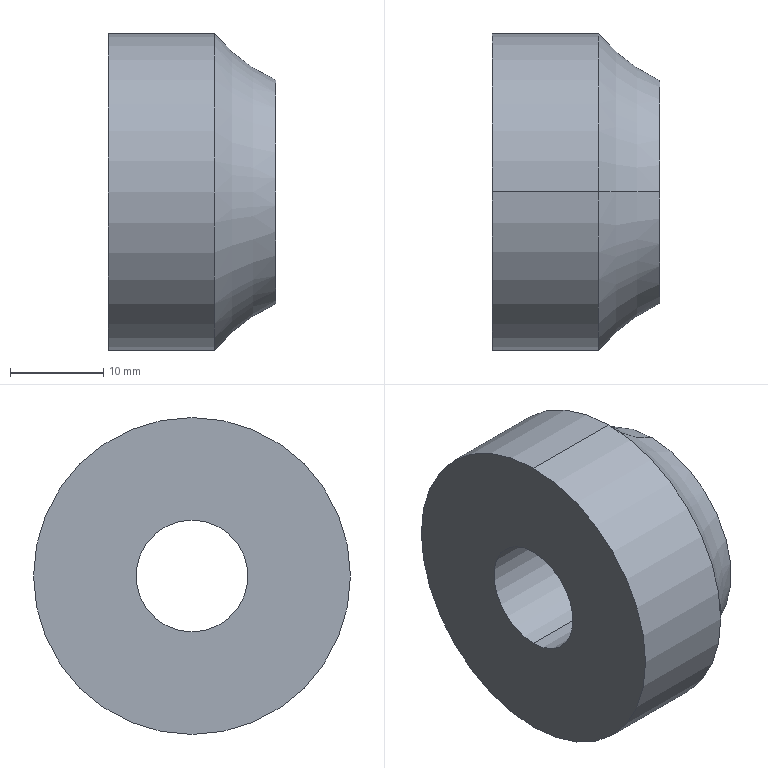Part | SolidWorks | features ICE 1, Revolution 1 | 1 solid | 8 faces | box 18 x 34 x 34 mm | volume 12469 mm3 | cylinder 4 | torus 2 | plane 2 | commonest cylinder face diameters 12 x2 34 x2
STEP:
#1=CARTESIAN_POINT('',(0.,0.,6.));
#2=VERTEX_POINT('',#1);
#3=CARTESIAN_POINT('',(0.,0.,-6.));
#4=VERTEX_POINT('',#3);
#5=CARTESIAN_POINT('',(0.,0.,0.));
#6=DIRECTION('',(1.,0.,0.));
#7=DIRECTION('',(0.,0.,-1.));
#8=AXIS2_PLACEMENT_3D('',#5,#6,#7);
#9=CIRCLE('',#8,6.);
#10=EDGE_CURVE('',#2,#4,#9,.T.);
#11=ORIENTED_EDGE('',*,*,#10,.F.);
#12=CARTESIAN_POINT('',(18.,0.,6.));
#13=VERTEX_POINT('',#12);
#14=CARTESIAN_POINT('',(0.,0.,6.));
#15=DIRECTION('',(1.,0.,0.));
#16=VECTOR('',#15,1000.);
#17=LINE('',#14,#16);
#18=EDGE_CURVE('',#2,#13,#17,.T.);
#19=ORIENTED_EDGE('',*,*,#18,.T.);
#20=CARTESIAN_POINT('',(18.,0.,-6.));
#21=VERTEX_POINT('',#20);
#22=CARTESIAN_POINT('',(18.,0.,0.));
#23=DIRECTION('',(-1.,0.,0.));
#24=DIRECTION('',(0.,0.,1.));
#25=AXIS2_PLACEMENT_3D('',#22,#23,#24);
#26=CIRCLE('',#25,6.);
#27=EDGE_CURVE('',#21,#13,#26,.T.);
#28=ORIENTED_EDGE('',*,*,#27,.F.);
#29=CARTESIAN_POINT('',(0.,0.,-6.));
#30=DIRECTION('',(1.,0.,0.));
#31=VECTOR('',#30,1000.);
#32=LINE('',#29,#31);
#33=EDGE_CURVE('',#4,#21,#32,.T.);
#34=ORIENTED_EDGE('',*,*,#33,.F.);
#35=EDGE_LOOP('',(#11,#19,#28,#34));
#36=FACE_OUTER_BOUND('',#35,.T.);
#37=CARTESIAN_POINT('',(0.,0.,0.));
#38=DIRECTION('',(1.,0.,0.));
#39=DIRECTION('',(0.,0.,-1.));
#40=AXIS2_PLACEMENT_3D('',#37,#38,#39);
#41=CYLINDRICAL_SURFACE('',#40,6.);
#42=ADVANCED_FACE('',(#36),#41,.F.);
#43=CARTESIAN_POINT('',(11.4,0.,17.));
#44=VERTEX_POINT('',#43);
#45=CARTESIAN_POINT('',(11.4,0.,-17.));
#46=VERTEX_POINT('',#45);
#47=CARTESIAN_POINT('',(11.4,0.,0.));
#48=DIRECTION('',(-1.,0.,0.));
#49=DIRECTION('',(0.,0.,1.));
#50=AXIS2_PLACEMENT_3D('',#47,#48,#49);
#51=CIRCLE('',#50,17.);
#52=EDGE_CURVE('',#44,#46,#51,.T.);
#53=ORIENTED_EDGE('',*,*,#52,.T.);
#54=CARTESIAN_POINT('',(0.,0.,-17.));
#55=VERTEX_POINT('',#54);
#56=CARTESIAN_POINT('',(0.,0.,-17.));
#57=DIRECTION('',(-1.,0.,0.));
#58=VECTOR('',#57,1000.);
#59=LINE('',#56,#58);
#60=EDGE_CURVE('',#46,#55,#59,.T.);
#61=ORIENTED_EDGE('',*,*,#60,.T.);
#62=CARTESIAN_POINT('',(0.,0.,17.));
#63=VERTEX_POINT('',#62);
#64=CARTESIAN_POINT('',(0.,0.,0.));
#65=DIRECTION('',(-1.,0.,0.));
#66=DIRECTION('',(0.,0.,1.));
#67=AXIS2_PLACEMENT_3D('',#64,#65,#66);
#68=CIRCLE('',#67,17.);
#69=EDGE_CURVE('',#63,#55,#68,.T.);
#70=ORIENTED_EDGE('',*,*,#69,.F.);
#71=CARTESIAN_POINT('',(0.,0.,17.));
#72=DIRECTION('',(-1.,0.,0.));
#73=VECTOR('',#72,1000.);
#74=LINE('',#71,#73);
#75=EDGE_CURVE('',#44,#63,#74,.T.);
#76=ORIENTED_EDGE('',*,*,#75,.F.);
#77=EDGE_LOOP('',(#53,#61,#70,#76));
#78=FACE_OUTER_BOUND('',#77,.T.);
#79=CARTESIAN_POINT('',(0.,0.,0.));
#80=DIRECTION('',(-1.,0.,0.));
#81=DIRECTION('',(0.,0.,1.));
#82=AXIS2_PLACEMENT_3D('',#79,#80,#81);
#83=CYLINDRICAL_SURFACE('',#82,17.);
#84=ADVANCED_FACE('',(#78),#83,.T.);
#85=CARTESIAN_POINT('',(11.4,0.,0.));
#86=DIRECTION('',(-1.,0.,0.));
#87=DIRECTION('',(0.,0.,1.));
#88=AXIS2_PLACEMENT_3D('',#85,#86,#87);
#89=CIRCLE('',#88,17.);
#90=EDGE_CURVE('',#46,#44,#89,.T.);
#91=ORIENTED_EDGE('',*,*,#90,.F.);
#92=CARTESIAN_POINT('',(18.,0.,-12.));
#93=VERTEX_POINT('',#92);
#94=CARTESIAN_POINT('',(24.968,0.,-28.053));
#95=DIRECTION('',(0.,1.,0.));
#96=DIRECTION('',(0.,0.,1.));
#97=AXIS2_PLACEMENT_3D('',#94,#95,#96);
#98=CIRCLE('',#97,17.5);
#99=EDGE_CURVE('',#46,#93,#98,.T.);
#100=ORIENTED_EDGE('',*,*,#99,.T.);
#101=CARTESIAN_POINT('',(18.,0.,12.));
#102=VERTEX_POINT('',#101);
#103=CARTESIAN_POINT('',(18.,0.,0.));
#104=DIRECTION('',(-1.,0.,0.));
#105=DIRECTION('',(0.,0.,1.));
#106=AXIS2_PLACEMENT_3D('',#103,#104,#105);
#107=CIRCLE('',#106,12.);
#108=EDGE_CURVE('',#93,#102,#107,.T.);
#109=ORIENTED_EDGE('',*,*,#108,.T.);
#110=CARTESIAN_POINT('',(24.968,0.,28.053));
#111=DIRECTION('',(0.,-1.,0.));
#112=DIRECTION('',(0.,0.,-1.));
#113=AXIS2_PLACEMENT_3D('',#110,#111,#112);
#114=CIRCLE('',#113,17.5);
#115=EDGE_CURVE('',#44,#102,#114,.T.);
#116=ORIENTED_EDGE('',*,*,#115,.F.);
#117=EDGE_LOOP('',(#91,#100,#109,#116));
#118=FACE_OUTER_BOUND('',#117,.T.);
#119=CARTESIAN_POINT('',(24.968,0.,0.));
#120=DIRECTION('',(-1.,0.,0.));
#121=DIRECTION('',(0.,0.,1.));
#122=AXIS2_PLACEMENT_3D('',#119,#120,#121);
#123=TOROIDAL_SURFACE('',#122,28.053,17.5);
#124=ADVANCED_FACE('',(#118),#123,.F.);
#125=ORIENTED_EDGE('',*,*,#27,.T.);
#126=CARTESIAN_POINT('',(18.,0.,0.));
#127=DIRECTION('',(-1.,0.,0.));
#128=DIRECTION('',(0.,0.,1.));
#129=AXIS2_PLACEMENT_3D('',#126,#127,#128);
#130=CIRCLE('',#129,6.);
#131=EDGE_CURVE('',#13,#21,#130,.T.);
#132=ORIENTED_EDGE('',*,*,#131,.T.);
#133=EDGE_LOOP('',(#125,#132));
#134=FACE_BOUND('',#133,.T.);
#135=CARTESIAN_POINT('',(18.,0.,0.));
#136=DIRECTION('',(-1.,0.,0.));
#137=DIRECTION('',(0.,0.,1.));
#138=AXIS2_PLACEMENT_3D('',#135,#136,#137);
#139=CIRCLE('',#138,12.);
#140=EDGE_CURVE('',#102,#93,#139,.T.);
#141=ORIENTED_EDGE('',*,*,#140,.F.);
#142=ORIENTED_EDGE('',*,*,#108,.F.);
#143=EDGE_LOOP('',(#141,#142));
#144=FACE_OUTER_BOUND('',#143,.T.);
#145=CARTESIAN_POINT('',(18.,12.,0.));
#146=DIRECTION('',(-1.,0.,0.));
#147=DIRECTION('',(0.,0.,1.));
#148=AXIS2_PLACEMENT_3D('',#145,#146,#147);
#149=PLANE('',#148);
#150=ADVANCED_FACE('',(#134,#144),#149,.F.);
#151=ORIENTED_EDGE('',*,*,#99,.F.);
#152=ORIENTED_EDGE('',*,*,#52,.F.);
#153=ORIENTED_EDGE('',*,*,#115,.T.);
#154=ORIENTED_EDGE('',*,*,#140,.T.);
#155=EDGE_LOOP('',(#151,#152,#153,#154));
#156=FACE_OUTER_BOUND('',#155,.T.);
#157=CARTESIAN_POINT('',(24.968,0.,0.));
#158=DIRECTION('',(-1.,0.,0.));
#159=DIRECTION('',(0.,0.,1.));
#160=AXIS2_PLACEMENT_3D('',#157,#158,#159);
#161=TOROIDAL_SURFACE('',#160,28.053,17.5);
#162=ADVANCED_FACE('',(#156),#161,.F.);
#163=ORIENTED_EDGE('',*,*,#60,.F.);
#164=ORIENTED_EDGE('',*,*,#90,.T.);
#165=ORIENTED_EDGE('',*,*,#75,.T.);
#166=CARTESIAN_POINT('',(0.,0.,0.));
#167=DIRECTION('',(-1.,0.,0.));
#168=DIRECTION('',(0.,0.,1.));
#169=AXIS2_PLACEMENT_3D('',#166,#167,#168);
#170=CIRCLE('',#169,17.);
#171=EDGE_CURVE('',#55,#63,#170,.T.);
#172=ORIENTED_EDGE('',*,*,#171,.F.);
#173=EDGE_LOOP('',(#163,#164,#165,#172));
#174=FACE_OUTER_BOUND('',#173,.T.);
#175=CARTESIAN_POINT('',(0.,0.,0.));
#176=DIRECTION('',(-1.,0.,0.));
#177=DIRECTION('',(0.,0.,1.));
#178=AXIS2_PLACEMENT_3D('',#175,#176,#177);
#179=CYLINDRICAL_SURFACE('',#178,17.);
#180=ADVANCED_FACE('',(#174),#179,.T.);
#181=CARTESIAN_POINT('',(0.,0.,0.));
#182=DIRECTION('',(1.,0.,0.));
#183=DIRECTION('',(0.,0.,-1.));
#184=AXIS2_PLACEMENT_3D('',#181,#182,#183);
#185=CIRCLE('',#184,6.);
#186=EDGE_CURVE('',#4,#2,#185,.T.);
#187=ORIENTED_EDGE('',*,*,#186,.T.);
#188=ORIENTED_EDGE('',*,*,#10,.T.);
#189=EDGE_LOOP('',(#187,#188));
#190=FACE_BOUND('',#189,.T.);
#191=ORIENTED_EDGE('',*,*,#69,.T.);
#192=ORIENTED_EDGE('',*,*,#171,.T.);
#193=EDGE_LOOP('',(#191,#192));
#194=FACE_OUTER_BOUND('',#193,.T.);
#195=CARTESIAN_POINT('',(0.,0.,0.));
#196=DIRECTION('',(1.,0.,0.));
#197=DIRECTION('',(0.,0.,-1.));
#198=AXIS2_PLACEMENT_3D('',#195,#196,#197);
#199=PLANE('',#198);
#200=ADVANCED_FACE('',(#190,#194),#199,.F.);
#201=ORIENTED_EDGE('',*,*,#18,.F.);
#202=ORIENTED_EDGE('',*,*,#186,.F.);
#203=ORIENTED_EDGE('',*,*,#33,.T.);
#204=ORIENTED_EDGE('',*,*,#131,.F.);
#205=EDGE_LOOP('',(#201,#202,#203,#204));
#206=FACE_OUTER_BOUND('',#205,.T.);
#207=CARTESIAN_POINT('',(0.,0.,0.));
#208=DIRECTION('',(1.,0.,0.));
#209=DIRECTION('',(0.,0.,-1.));
#210=AXIS2_PLACEMENT_3D('',#207,#208,#209);
#211=CYLINDRICAL_SURFACE('',#210,6.);
#212=ADVANCED_FACE('',(#206),#211,.F.);
#213=CLOSED_SHELL('',(#42,#84,#124,#150,#162,#180,#200,#212));
#214=MANIFOLD_SOLID_BREP('',#213);
#215=CARTESIAN_POINT('',(0.,0.,0.));
#216=DIRECTION('',(0.,0.,1.));
#217=DIRECTION('',(1.,0.,0.));
#218=AXIS2_PLACEMENT_3D('',#215,#216,#217);
#219=(LENGTH_UNIT()NAMED_UNIT(*)SI_UNIT(.MILLI.,.METRE.));
#220=UNCERTAINTY_MEASURE_WITH_UNIT(LENGTH_MEASURE(0.00001),#219,'','');
#221=(NAMED_UNIT(*)PLANE_ANGLE_UNIT()SI_UNIT($,.RADIAN.));
#222=(NAMED_UNIT(*)SI_UNIT($,.STERADIAN.)SOLID_ANGLE_UNIT());
#223=(GEOMETRIC_REPRESENTATION_CONTEXT(3)GLOBAL_UNCERTAINTY_ASSIGNED_CONTEXT((#220))GLOBAL_UNIT_ASSIGNED_CONTEXT((#219,#221,#222))REPRESENTATION_CONTEXT('',''));
#224=ADVANCED_BREP_SHAPE_REPRESENTATION('',(#214,#218),#223);